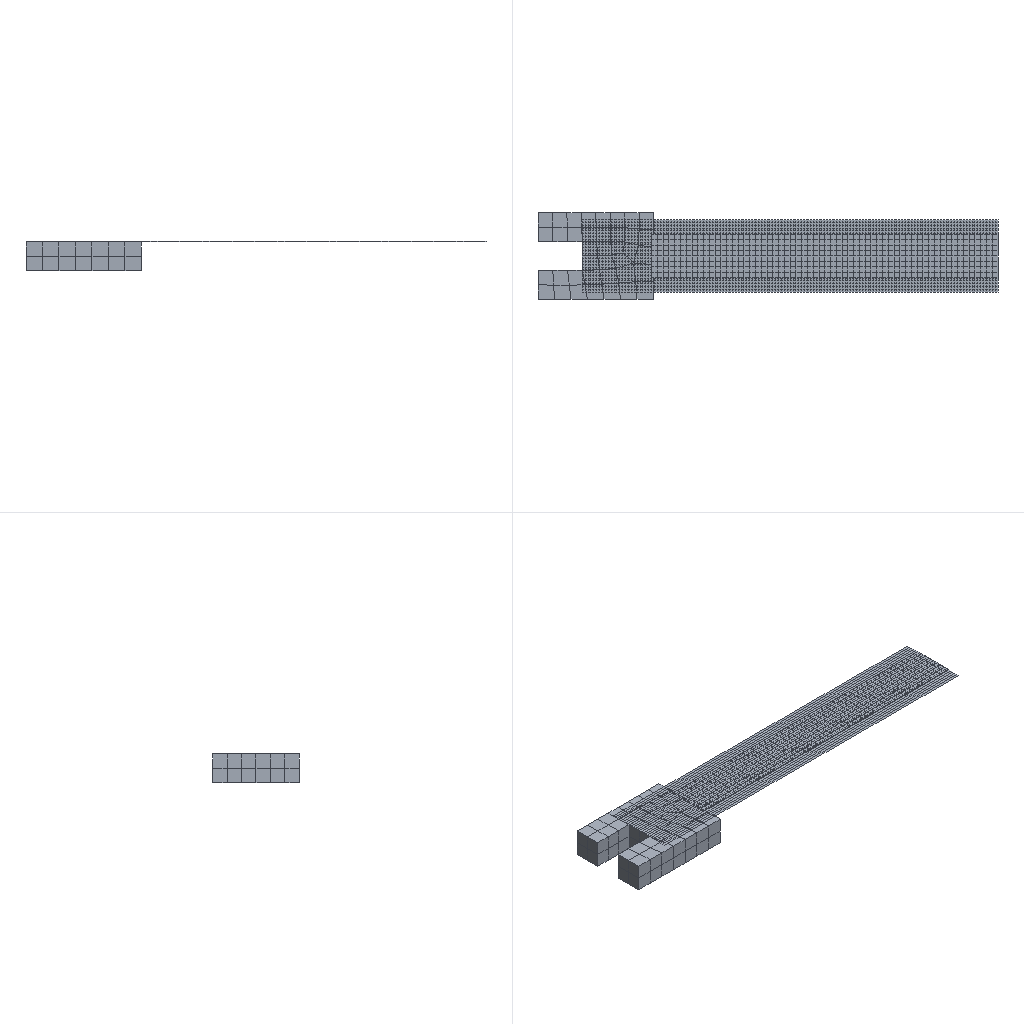Simulation study | abaqus
Set-up summary:
category,name,step,type,value,unit,region
solver,abaqus
solver,version,,,Abaqus/Standard 2020
units,not stated in the deck,,not stated
analysis,deck,,transient,transient
load_step,Step-1,Step-1,transient,nlgeom=True
load_step,Step-2,Step-2,transient,nlgeom=True
contact,interactions,,,general=0 pairs=0 ties=2
load_step,requested,,,2
mesh,nodes,,,5179
mesh,elements,,,4300
element_type,S4R,,shell,3744
element_type,C3D8E,,solid,480
element_type,C3D8R,,solid,76
load,load commands in deck,,count,4
bc,support commands in deck,,count,28
material,MATERIAL-1,,in results
material,MATERIAL-PZT,,in results
check,setup vs results,,match,"per instance, exact: element labels, types and connectivity; labels of the nodes the elements use; coordinates of those nodes at SINGLE_PRECISION in 3 of 3 instance(s)"
Abaqus input file, long lists of numbers shortened:
*Heading
** Job name: Job-1 Model name: Job-18
** Generated by: Abaqus/CAE 2020
*Preprint, echo=NO, model=NO, history=NO, contact=NO
**
** PARTS
**
*Part, name=STEEL
*Node
      1,         144.,         3.75,           0.
      2,           0.,         3.75,           0.
** (3913 more lines like these left out)
*Element, type=S4R
   1,    1,    7,  484,  316
   2,    7,    8,  485,  484
** (3742 more lines like these left out)
*Nset, nset=SET-1, generate
    1,  3915,     1
*Elset, elset=SET-1, generate
    1,  3744,     1
** Section: Section-3-SET-1
*Shell Section, elset=SET-1, material=MATERIAL-1
0.1, 5
*End Part
**
*Part, name=WORK-3
*Node
      1,   73.129,   18.935,   10.2
      2,   73.129,   17.06,   10.2
** (1096 more lines like these left out)
*Element, type=C3D8E
  1,   19,   20,   29,   28,    1,    2,   11,   10
  2,   20,   21,   30,   29,    2,    3,   12,   11
** (478 more lines like these left out)
*Nset, nset=Set-2, generate
    1,  1098,     1
*Elset, elset=Set-2, generate
   1,  480,    1
*Nset, nset=Set-3, generate
    1,  1098,     1
*Elset, elset=Set-3, generate
   1,  480,    1
*Orientation, name=Ori-1
1., 0., 0., 0., 1., 0.
1, 0.
** Section: Section-4
*Solid Section, elset=Set-3, orientation=Ori-1, material=MATERIAL-PZT
,
*End Part
**
*Part, name="lianjie jiaju fnagzhen"
*Node
      1,  -46.219,    26.435,           0.
      2,  -86.219,    26.435,           0.
** (164 more lines like these left out)
*Element, type=C3D8R
 1,   2,  32,  35,   9,  57,  87,  90,  64
 2,   8,  30,  35,  32,  63,  85,  90,  87
** (74 more lines like these left out)
*Nset, nset="lianjie jiaju fnagzhen-RefPt_", internal
 166,
*Nset, nset=SET-1, generate
   1,  165,    1
*Elset, elset=SET-1, generate
  1,  76,   1
** Section: Section-2-SET-1
*Solid Section, elset=SET-1, material=MATERIAL-1
,
*End Part
**
**
** ASSEMBLY
**
*Assembly, name=Assembly
**
*Instance, name=STEEL-1, part=STEEL
  -70.871,     7.685,          10.
*End Instance
**
*Instance, name="lianjie jiaju fnagzhen-1", part="lianjie jiaju fnagzhen"
*End Instance
**
*Instance, name=WORK-3-1, part=WORK-3
*End Instance
**
*Node
      1,  -70.871,   11.435,           5.
      2,  -70.871,   11.435,           5.
*Nset, nset=B_SET-1, instance="lianjie jiaju fnagzhen-1", generate
   1,  165,    1
*Elset, elset=B_SET-1, instance="lianjie jiaju fnagzhen-1", generate
  1,  76,   1
*Nset, nset=M_SET-7, instance="lianjie jiaju fnagzhen-1"
 166,
*Nset, nset=M_SET-8, instance="lianjie jiaju fnagzhen-1"
 166,
*Nset, nset=M_SET-9, instance="lianjie jiaju fnagzhen-1"
 166,
*Nset, nset=SET-5, instance="lianjie jiaju fnagzhen-1"
 61, 62, 84
*Elset, elset=SET-5, instance="lianjie jiaju fnagzhen-1"
 11, 23, 49, 61
*Nset, nset=SET-8, instance="lianjie jiaju fnagzhen-1"
 84,
*Nset, nset=SET-11, instance=STEEL-1
   1,   2,   7,   8,   9,  10,  11,  12,  13,  14,  15,  16,  17,  18,  19,  20
  21,  22,  23,  24,  25,  26,  27,  28,  29,  30,  31,  32,  33,  34,  35,  36
** (8 more lines like these left out)
*Elset, elset=SET-11, instance=STEEL-1
    1,    2,    3,    4,    5,    6,    7,    8,    9,   10,   11,   12,   13,   14,   15,   16
   17,   18,   19,   20,   21,   22,   23,   24,   25,   26,   27,   28,   29,   30,   31,   32
** (16 more lines like these left out)
*Nset, nset=SET-12, instance=STEEL-1
   1,   4, 305, 306, 307, 308, 309, 310, 311, 312, 313, 314, 315, 316
*Elset, elset=SET-12, instance=STEEL-1, generate
    1,  1729,   144
*Nset, nset=SET-13, instance=STEEL-1
   1,   5, 317, 318, 319, 320, 321, 322, 323, 324, 325, 326, 327, 328
*Elset, elset=SET-13, instance=STEEL-1, generate
 2016,  3744,   144
*Nset, nset=Set-23, instance=WORK-3-1, generate
  1,  18,   1
*Elset, elset=Set-23, instance=WORK-3-1, generate
 1,  8,  1
*Elset, elset="_CP-1-lianjie jiaju fnagzhen-1_S2", internal, instance="lianjie jiaju fnagzhen-1", generate
 39,  76,   1
*Elset, elset=_CP-2-STEEL-1_SNEG, internal, instance=STEEL-1, generate
    1,  3744,     1
*Elset, elset="_CP-2-lianjie jiaju fnagzhen-1_S2", internal, instance="lianjie jiaju fnagzhen-1", generate
 39,  76,   1
*Elset, elset=_CP-4-STEEL-1_SPOS, internal, instance=STEEL-1, generate
    1,  3744,     1
*Nset, nset=_PICKEDSET7, internal, instance="lianjie jiaju fnagzhen-1"
 166,
*Nset, nset=_PickedSet44, internal, instance="lianjie jiaju fnagzhen-1"
 166,
*Elset, elset=_S_SURF-3_S4, internal, instance="lianjie jiaju fnagzhen-1"
 61,
*Elset, elset=_S_SURF-3_S6, internal, instance="lianjie jiaju fnagzhen-1"
 49,
*Elset, elset=_S_SURF-4_S4, internal, instance="lianjie jiaju fnagzhen-1"
 61,
*Elset, elset=_S_SURF-4_S6, internal, instance="lianjie jiaju fnagzhen-1"
 49,
*Elset, elset=_S_SURF-5_S4, internal, instance="lianjie jiaju fnagzhen-1"
 61,
*Elset, elset=_S_SURF-5_S6, internal, instance="lianjie jiaju fnagzhen-1"
 49,
*Elset, elset="_CP-1-lianjie jiaju fnagzhen-1_S2", internal, instance="lianjie jiaju fnagzhen-1", generate
 39,  76,   1
*Surface, type=ELEMENT, name="CP-1-lianjie jiaju fnagzhen-1"
"_CP-1-lianjie jiaju fnagzhen-1_S2", S2
*Surface, type=ELEMENT, name=CP-2-STEEL-1
_CP-2-STEEL-1_SNEG, SNEG
*Elset, elset="_CP-2-lianjie jiaju fnagzhen-1_S2", internal, instance="lianjie jiaju fnagzhen-1", generate
 39,  76,   1
*Surface, type=ELEMENT, name="CP-2-lianjie jiaju fnagzhen-1"
"_CP-2-lianjie jiaju fnagzhen-1_S2", S2
*Surface, type=ELEMENT, name=CP-4-STEEL-1
_CP-4-STEEL-1_SPOS, SPOS
*Elset, elset=_S_SURF-3_S6_1, internal, instance="lianjie jiaju fnagzhen-1"
 49,
*Elset, elset=_S_SURF-3_S4_1, internal, instance="lianjie jiaju fnagzhen-1"
 61,
*Surface, type=ELEMENT, name=S_SURF-3
_S_SURF-3_S6_1, S6
_S_SURF-3_S4_1, S4
*Elset, elset=_S_SURF-4_S6_1, internal, instance="lianjie jiaju fnagzhen-1"
 49,
*Elset, elset=_S_SURF-4_S4_1, internal, instance="lianjie jiaju fnagzhen-1"
 61,
*Surface, type=ELEMENT, name=S_SURF-4
_S_SURF-4_S6_1, S6
_S_SURF-4_S4_1, S4
*Elset, elset=_S_SURF-5_S6_1, internal, instance="lianjie jiaju fnagzhen-1"
 49,
*Elset, elset=_S_SURF-5_S4_1, internal, instance="lianjie jiaju fnagzhen-1"
 61,
*Surface, type=ELEMENT, name=S_SURF-5
_S_SURF-5_S6_1, S6
_S_SURF-5_S4_1, S4
*Elset, elset=_s_Surf-9_S5, internal, instance=WORK-3-1, generate
   1,  480,    1
*Surface, type=ELEMENT, name=s_Surf-9
_s_Surf-9_S5, S5
** Constraint: CONSTRAINT-3
*Coupling, constraint name=CONSTRAINT-3, ref node=M_SET-9, surface=S_SURF-5
*Kinematic
** Constraint: CP-1-lianjie jiaju fnagzhen-1-steel-1-1
*Tie, name="CP-1-lianjie jiaju fnagzhen-1-steel-1-1", adjust=yes, type=SURFACE TO SURFACE
CP-2-STEEL-1, "CP-2-lianjie jiaju fnagzhen-1"
** Constraint: CP-3-STEEL-1-PART-3-1-1
*Tie, name=CP-3-STEEL-1-PART-3-1-1, adjust=yes, type=SURFACE TO SURFACE
s_Surf-9, CP-4-STEEL-1
** Constraint: RigidBody-1
*Rigid Body, ref node=_PickedSet44, elset=B_SET-1
*End Assembly
*Amplitude, name=AMP-1
             0.,              0.,             0.5,              1.
*Amplitude, name=AMP-2
             0.,              0.,              1.,              1.
**
** MATERIALS
**
*Material, name=MATERIAL-1
*Density
 7.85e-09,
*Elastic
197000., 0.23
*Material, name=MATERIAL-PZT
*Density
 1.78e-09,
*Dielectric, type=ANISO
 8.4115e-09,         0., 8.4115e-09,         0.,         0., 9.2969e-09
*Elastic
2400., 0.35
*Piezoelectric, type=E
0.,        0.,        0.,        0.,  1.08e-11,        0.,        0.,        0.
        0.,  1.08e-11,        0.,        0., -1.73e-11, -1.73e-11,   2.1e-11,        0.
        0.,        0.
**
** BOUNDARY CONDITIONS
**
** Name: Disp-BC-1 Type: 位移/转角
*Boundary
SET-12, 1, 1
** Name: Disp-BC-2 Type: 位移/转角
*Boundary
SET-12, 2, 2
** Name: Disp-BC-3 Type: 位移/转角
*Boundary
SET-12, 3, 3
** Name: Disp-BC-4 Type: 位移/转角
*Boundary
SET-13, 1, 1
** Name: Disp-BC-5 Type: 位移/转角
*Boundary
SET-13, 2, 2
** Name: Disp-BC-6 Type: 位移/转角
*Boundary
SET-13, 3, 3
** ----------------------------------------------------------------
**
** STEP: Step-1
**
*Step, name=Step-1, nlgeom=YES
*Dynamic,application=QUASI-STATIC,initial=NO
1.,1.,1e-05
**
** BOUNDARY CONDITIONS
**
** Name: BC-28 Type: 电势
*Boundary, op=NEW
Set-23, 9, 9
** Name: Disp-BC-1 Type: 位移/转角
*Boundary, op=NEW
** Name: Disp-BC-2 Type: 位移/转角
*Boundary, op=NEW
** Name: Disp-BC-3 Type: 位移/转角
*Boundary, op=NEW
** Name: Disp-BC-4 Type: 位移/转角
*Boundary, op=NEW
** Name: Disp-BC-5 Type: 位移/转角
*Boundary, op=NEW
** Name: Disp-BC-6 Type: 位移/转角
*Boundary, op=NEW
** Name: Disp-BC-7 Type: 位移/转角
*Boundary, op=NEW, amplitude=AMP-1
SET-12, 1, 1
** Name: Disp-BC-8 Type: 位移/转角
*Boundary, op=NEW, amplitude=AMP-1
SET-12, 2, 2
** Name: Disp-BC-9 Type: 位移/转角
*Boundary, op=NEW, amplitude=AMP-1
SET-12, 3, 3
** Name: Disp-BC-10 Type: 位移/转角
*Boundary, op=NEW, amplitude=AMP-1
SET-12, 5, 5, -0.08727
** Name: Disp-BC-11 Type: 位移/转角
*Boundary, op=NEW, amplitude=AMP-2
SET-5, 2, 2
** Name: Disp-BC-12 Type: 位移/转角
*Boundary, op=NEW, amplitude=AMP-2
SET-5, 3, 3
** Name: Disp-BC-13 Type: 位移/转角
*Boundary, op=NEW, amplitude=AMP-2
SET-5, 5, 5
** Name: Disp-BC-14 Type: 位移/转角
*Boundary, op=NEW, amplitude=AMP-1
SET-13, 1, 1
** Name: Disp-BC-15 Type: 位移/转角
*Boundary, op=NEW, amplitude=AMP-1
SET-13, 2, 2
** Name: Disp-BC-16 Type: 位移/转角
*Boundary, op=NEW, amplitude=AMP-1
SET-13, 3, 3
** Name: Disp-BC-17 Type: 位移/转角
*Boundary, op=NEW, amplitude=AMP-1
SET-13, 5, 5, -0.08727
**
** OUTPUT REQUESTS
**
*Restart, write, frequency=0
**
** FIELD OUTPUT: F-Output-5
**
*Output, field
*Node Output
CECHG, CECUR, EPOT, RCHG, RECUR
*Element Output, directions=YES
ECD, EFLX, EPG, NCURS
*Contact Output
ECD, ECDA, ECDT, ECDTA
**
** FIELD OUTPUT: F-Output-1
**
*Output, field, variable=PRESELECT
**
** HISTORY OUTPUT: H-Output-1
**
*Output, history, variable=PRESELECT, frequency=1
*End Step
** ----------------------------------------------------------------
**
** STEP: Step-2
**
*Step, name=Step-2, nlgeom=YES, inc=100000
*Dynamic,application=QUASI-STATIC,initial=NO
0.01,1.,1e-05
**
** BOUNDARY CONDITIONS
**
** Name: BC-28 Type: 电势
*Boundary, op=NEW
Set-23, 9, 9
** Name: Disp-BC-7 Type: 位移/转角
*Boundary, op=NEW
** Name: Disp-BC-8 Type: 位移/转角
*Boundary, op=NEW
** Name: Disp-BC-9 Type: 位移/转角
*Boundary, op=NEW
** Name: Disp-BC-10 Type: 位移/转角
*Boundary, op=NEW
** Name: Disp-BC-11 Type: 位移/转角
*Boundary, op=NEW
** Name: Disp-BC-12 Type: 位移/转角
*Boundary, op=NEW
** Name: Disp-BC-13 Type: 位移/转角
*Boundary, op=NEW
** Name: Disp-BC-14 Type: 位移/转角
*Boundary, op=NEW
** Name: Disp-BC-15 Type: 位移/转角
*Boundary, op=NEW
** Name: Disp-BC-16 Type: 位移/转角
*Boundary, op=NEW
** Name: Disp-BC-17 Type: 位移/转角
*Boundary, op=NEW
** Name: Disp-BC-18 Type: 位移/转角
*Boundary, op=NEW, amplitude=AMP-2
SET-12, 1, 1
** Name: Disp-BC-19 Type: 位移/转角
*Boundary, op=NEW, amplitude=AMP-2
SET-12, 2, 2
** Name: Disp-BC-20 Type: 位移/转角
*Boundary, op=NEW, amplitude=AMP-2
SET-12, 3, 3
** Name: Disp-BC-21 Type: 位移/转角
*Boundary, op=NEW, amplitude=AMP-2
SET-5, 1, 1, 28.
** Name: Disp-BC-22 Type: 位移/转角
*Boundary, op=NEW, amplitude=AMP-2
SET-5, 2, 2
** Name: Disp-BC-23 Type: 位移/转角
*Boundary, op=NEW, amplitude=AMP-2
SET-5, 3, 3
** Name: Disp-BC-25 Type: 位移/转角
*Boundary, op=NEW, amplitude=AMP-2
SET-13, 1, 1
** Name: Disp-BC-26 Type: 位移/转角
*Boundary, op=NEW, amplitude=AMP-2
SET-13, 2, 2
** Name: Disp-BC-27 Type: 位移/转角
*Boundary, op=NEW, amplitude=AMP-2
SET-13, 3, 3
**
** LOADS
**
** Name: Load-1   Type: Moment
*Cload
M_SET-9, 5, -100.
**
** OUTPUT REQUESTS
**
*Restart, write, frequency=0
**
** FIELD OUTPUT: F-Output-2
**
*Output, field
*Node Output
A, CF, RF, RT, U, V
**
** FIELD OUTPUT: F-Output-4
**
*Contact Output
CDISP, CSTRESS
**
** FIELD OUTPUT: F-Output-5
**
*Node Output
CECHG, CECUR, EPOT, RCHG, RECUR
*Element Output, directions=YES
ECD, EFLX, EPG, NCURS
*Contact Output
ECD, ECDA, ECDT, ECDTA
**
** FIELD OUTPUT: F-Output-3
**
*Element Output, directions=YES
LE, PE, PEEQ, PEMAG, S
*Output, history, frequency=0
*End Step
Results summary:
result,step,,completed,increments=1 time=1.0/1.0
result,step,,completed,increments=96 time=1.0/1.0
result,analysis,,,transient
result,last_loadstep,,,2
result,analysis steps,,count,2
result,primary field,,,"U, UR"
result,reaction total,,FX,-8.5e-05,model units
result,reaction total,,FY,0.0,model units
result,reaction total,,FZ,-0.00017,model units